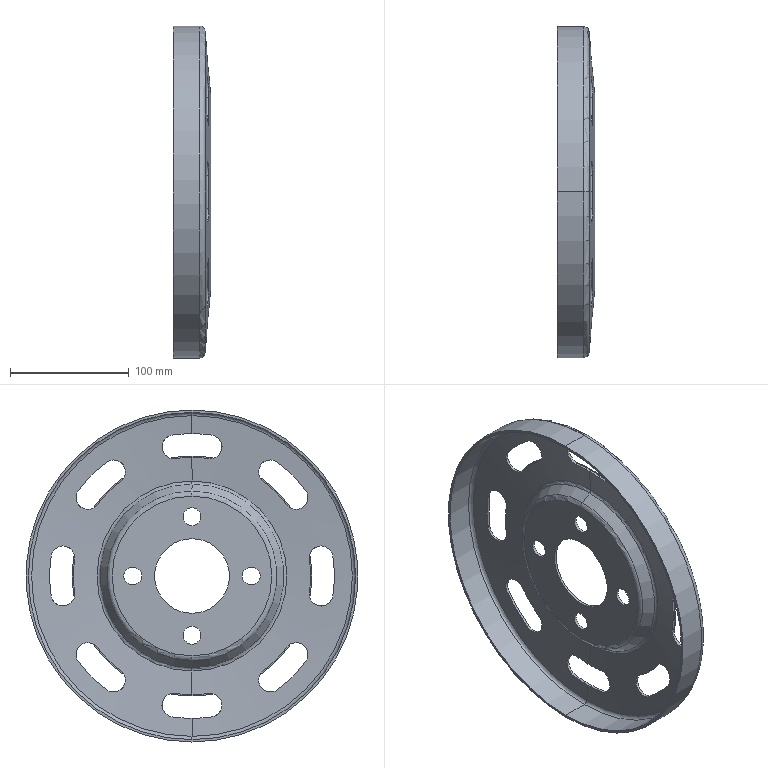Part | SolidWorks | features BaseBody 1 | 1 solid | 87 faces | box 31.836 x 280 x 280 mm | volume 146643 mm3 | cylinder 56 | torus 12 | plane 11 | cone 8 | commonest cylinder face diameters 20 x24 200 x9 240 x9 15 x8 63 x2 276 x2